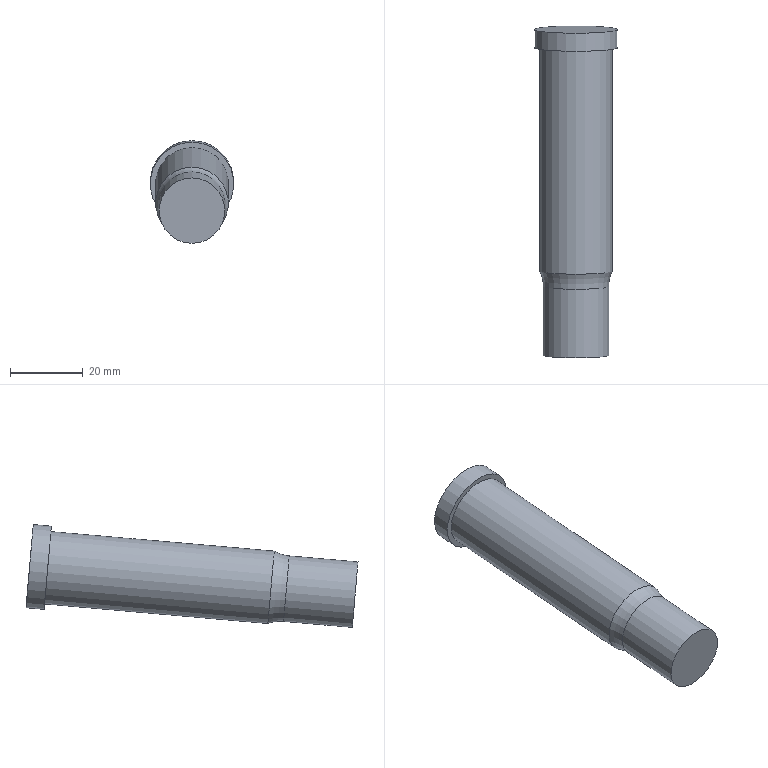Part | NX | features SPAS 20-80-18.10 2 | 1 solid | 7 faces | box 23 x 91.449 x 28.316 mm | volume 27536 mm3 | plane 3 | cylinder 3 | torus 1 | commonest cylinder face diameters 18.1 x1 20 x1 23 x1
STEP:
#1=CARTESIAN_POINT('',(147.466,50.681,-20.387));
#2=VERTEX_POINT('',#1);
#3=CARTESIAN_POINT('',(147.466,51.47,-29.402));
#4=DIRECTION('',(0.,0.9962,0.08716));
#5=DIRECTION('',(0.,-0.08716,0.9962));
#6=AXIS2_PLACEMENT_3D('',#3,#4,#5);
#7=CIRCLE('',#6,9.05);
#8=EDGE_CURVE('',#2,#2,#7,.T.);
#9=ORIENTED_EDGE('',*,*,#8,.F.);
#10=EDGE_LOOP('',(#9));
#11=FACE_BOUND('',#10,.T.);
#12=CARTESIAN_POINT('',(147.466,51.47,-29.402));
#13=DIRECTION('',(0.,-0.9962,-0.08716));
#14=DIRECTION('',(0.,0.08716,-0.9962));
#15=AXIS2_PLACEMENT_3D('',#12,#13,#14);
#16=PLANE('',#15);
#17=ADVANCED_FACE('',(#11),#16,.T.);
#18=CARTESIAN_POINT('',(147.466,69.609,-18.731));
#19=VERTEX_POINT('',#18);
#20=CARTESIAN_POINT('',(147.466,70.398,-27.746));
#21=DIRECTION('',(0.,0.9962,0.08716));
#22=DIRECTION('',(0.,-0.08716,0.9962));
#23=AXIS2_PLACEMENT_3D('',#20,#21,#22);
#24=CIRCLE('',#23,9.05);
#25=EDGE_CURVE('',#19,#19,#24,.F.);
#26=ORIENTED_EDGE('',*,*,#25,.T.);
#27=EDGE_LOOP('',(#26));
#28=FACE_BOUND('',#27,.T.);
#29=ORIENTED_EDGE('',*,*,#8,.T.);
#30=EDGE_LOOP('',(#29));
#31=FACE_BOUND('',#30,.T.);
#32=CARTESIAN_POINT('',(147.466,51.47,-29.402));
#33=DIRECTION('',(0.,0.9962,0.08716));
#34=DIRECTION('',(0.,-0.08716,0.9962));
#35=AXIS2_PLACEMENT_3D('',#32,#33,#34);
#36=CYLINDRICAL_SURFACE('',#35,9.05);
#37=ADVANCED_FACE('',(#28,#31),#36,.T.);
#38=CARTESIAN_POINT('',(147.466,137.018,-31.956));
#39=VERTEX_POINT('',#38);
#40=CARTESIAN_POINT('',(147.466,136.147,-21.994));
#41=DIRECTION('',(0.,-0.9962,-0.08716));
#42=DIRECTION('',(0.,0.08716,-0.9962));
#43=AXIS2_PLACEMENT_3D('',#40,#41,#42);
#44=CIRCLE('',#43,10.);
#45=EDGE_CURVE('',#39,#39,#44,.F.);
#46=ORIENTED_EDGE('',*,*,#45,.F.);
#47=EDGE_LOOP('',(#46));
#48=FACE_BOUND('',#47,.T.);
#49=CARTESIAN_POINT('',(147.466,73.764,-17.414));
#50=VERTEX_POINT('',#49);
#51=CARTESIAN_POINT('',(147.466,74.636,-27.376));
#52=DIRECTION('',(0.,0.9962,0.08716));
#53=DIRECTION('',(0.,-0.08716,0.9962));
#54=AXIS2_PLACEMENT_3D('',#51,#52,#53);
#55=CIRCLE('',#54,10.);
#56=EDGE_CURVE('',#50,#50,#55,.T.);
#57=ORIENTED_EDGE('',*,*,#56,.T.);
#58=EDGE_LOOP('',(#57));
#59=FACE_BOUND('',#58,.T.);
#60=CARTESIAN_POINT('',(147.466,74.636,-27.376));
#61=DIRECTION('',(0.,0.9962,0.08716));
#62=DIRECTION('',(0.,-0.08716,0.9962));
#63=AXIS2_PLACEMENT_3D('',#60,#61,#62);
#64=CYLINDRICAL_SURFACE('',#63,10.);
#65=ADVANCED_FACE('',(#48,#59),#64,.T.);
#66=CARTESIAN_POINT('',(147.466,140.125,-10.102));
#67=VERTEX_POINT('',#66);
#68=CARTESIAN_POINT('',(147.466,141.128,-21.558));
#69=DIRECTION('',(0.,0.9962,0.08716));
#70=DIRECTION('',(0.,-0.08716,0.9962));
#71=AXIS2_PLACEMENT_3D('',#68,#69,#70);
#72=CIRCLE('',#71,11.5);
#73=EDGE_CURVE('',#67,#67,#72,.F.);
#74=ORIENTED_EDGE('',*,*,#73,.F.);
#75=EDGE_LOOP('',(#74));
#76=FACE_BOUND('',#75,.T.);
#77=CARTESIAN_POINT('',(147.466,141.128,-21.558));
#78=DIRECTION('',(0.,0.9962,0.08716));
#79=DIRECTION('',(0.,-0.08716,0.9962));
#80=AXIS2_PLACEMENT_3D('',#77,#78,#79);
#81=PLANE('',#80);
#82=ADVANCED_FACE('',(#76),#81,.T.);
#83=ORIENTED_EDGE('',*,*,#45,.T.);
#84=EDGE_LOOP('',(#83));
#85=FACE_BOUND('',#84,.T.);
#86=CARTESIAN_POINT('',(147.466,137.149,-33.45));
#87=VERTEX_POINT('',#86);
#88=CARTESIAN_POINT('',(147.466,136.147,-21.994));
#89=DIRECTION('',(0.,-0.9962,-0.08716));
#90=DIRECTION('',(0.,0.08716,-0.9962));
#91=AXIS2_PLACEMENT_3D('',#88,#89,#90);
#92=CIRCLE('',#91,11.5);
#93=EDGE_CURVE('',#87,#87,#92,.F.);
#94=ORIENTED_EDGE('',*,*,#93,.F.);
#95=EDGE_LOOP('',(#94));
#96=FACE_BOUND('',#95,.T.);
#97=CARTESIAN_POINT('',(147.466,136.147,-21.994));
#98=DIRECTION('',(0.,-0.9962,-0.08716));
#99=DIRECTION('',(0.,0.08716,-0.9962));
#100=AXIS2_PLACEMENT_3D('',#97,#98,#99);
#101=PLANE('',#100);
#102=ADVANCED_FACE('',(#85,#96),#101,.T.);
#103=ORIENTED_EDGE('',*,*,#73,.T.);
#104=EDGE_LOOP('',(#103));
#105=FACE_BOUND('',#104,.T.);
#106=ORIENTED_EDGE('',*,*,#93,.T.);
#107=EDGE_LOOP('',(#106));
#108=FACE_BOUND('',#107,.T.);
#109=CARTESIAN_POINT('',(147.466,126.185,-22.866));
#110=DIRECTION('',(0.,0.9962,0.08716));
#111=DIRECTION('',(0.,-0.08716,0.9962));
#112=AXIS2_PLACEMENT_3D('',#109,#110,#111);
#113=CYLINDRICAL_SURFACE('',#112,11.5);
#114=ADVANCED_FACE('',(#105,#108),#113,.T.);
#115=ORIENTED_EDGE('',*,*,#25,.F.);
#116=EDGE_LOOP('',(#115));
#117=FACE_BOUND('',#116,.T.);
#118=ORIENTED_EDGE('',*,*,#56,.F.);
#119=EDGE_LOOP('',(#118));
#120=FACE_BOUND('',#119,.T.);
#121=CARTESIAN_POINT('',(147.466,70.398,-27.746));
#122=DIRECTION('',(0.,0.9962,0.08716));
#123=DIRECTION('',(0.,-0.08716,0.9962));
#124=AXIS2_PLACEMENT_3D('',#121,#122,#123);
#125=TOROIDAL_SURFACE('',#124,19.05,10.);
#126=ADVANCED_FACE('',(#117,#120),#125,.F.);
#127=CLOSED_SHELL('',(#17,#37,#65,#82,#102,#114,#126));
#128=MANIFOLD_SOLID_BREP('',#127);
#129=(LENGTH_UNIT()NAMED_UNIT(*)SI_UNIT(.MILLI.,.METRE.));
#130=UNCERTAINTY_MEASURE_WITH_UNIT(LENGTH_MEASURE(0.00001),#129,'','');
#131=(NAMED_UNIT(*)PLANE_ANGLE_UNIT()SI_UNIT($,.RADIAN.));
#132=(NAMED_UNIT(*)SI_UNIT($,.STERADIAN.)SOLID_ANGLE_UNIT());
#133=(GEOMETRIC_REPRESENTATION_CONTEXT(3)GLOBAL_UNCERTAINTY_ASSIGNED_CONTEXT((#130))GLOBAL_UNIT_ASSIGNED_CONTEXT((#129,#131,#132))REPRESENTATION_CONTEXT('',''));
#134=ADVANCED_BREP_SHAPE_REPRESENTATION('',(#128),#133);